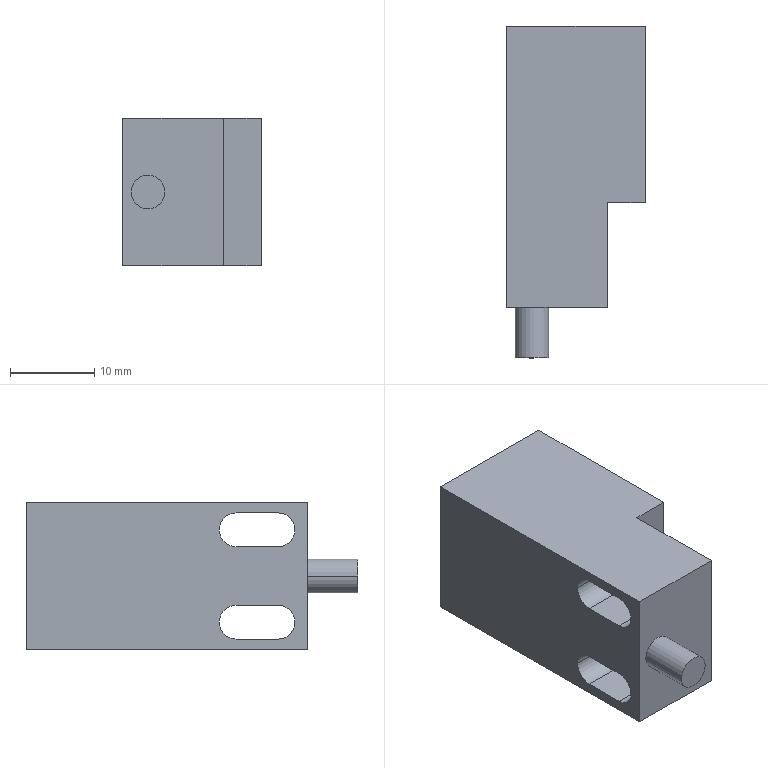Part | STEP file | 001-011-NPN10-30VDC | 1 solid | 21 faces | box 16.5 x 39.5 x 17.5 mm | volume 7983 mm3 | plane 13 | cylinder 8 | commonest cylinder face diameters 4 x8